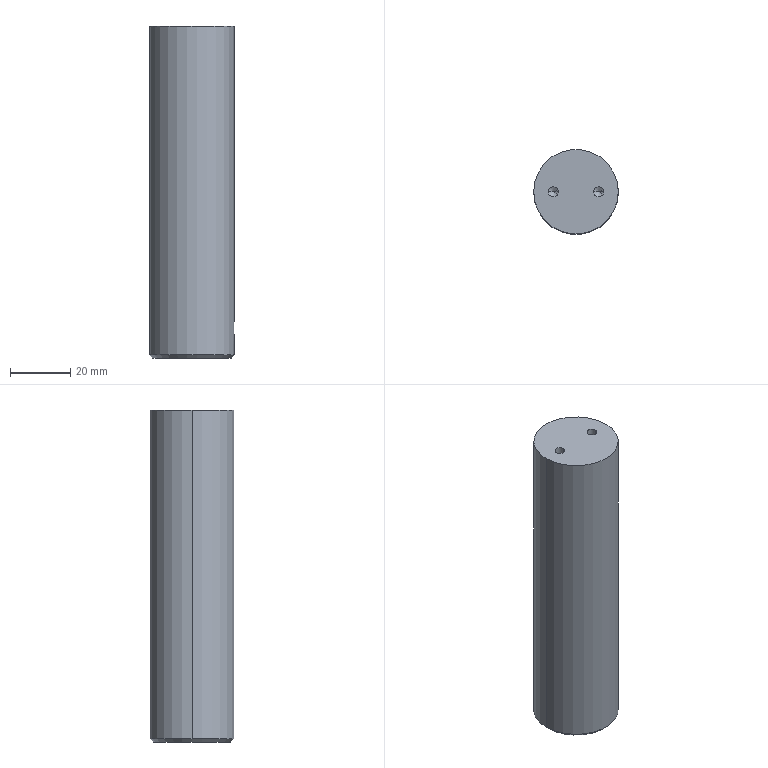Part | SolidWorks | features 3DProfileFeature 2, HoleWzd 2, Chamfer 1, Revolution 1 | 1 solid | 21 faces | box 28 x 28 x 110 mm | volume 51946 mm3 | cylinder 10 | cone 8 | plane 3 | commonest cylinder face diameters 3.3 x4 5 x2 18.1 x2 28 x2
STEP:
#1=CARTESIAN_POINT('',(9.05,0.,-109.));
#2=VERTEX_POINT('',#1);
#3=CARTESIAN_POINT('',(-9.05,0.,-109.));
#4=VERTEX_POINT('',#3);
#5=CARTESIAN_POINT('',(0.,0.,-109.));
#6=DIRECTION('',(0.,0.,-1.));
#7=DIRECTION('',(-1.,0.,0.));
#8=AXIS2_PLACEMENT_3D('',#5,#6,#7);
#9=CIRCLE('',#8,9.05);
#10=EDGE_CURVE('',#2,#4,#9,.T.);
#11=ORIENTED_EDGE('',*,*,#10,.F.);
#12=CARTESIAN_POINT('',(10.05,0.,-110.));
#13=VERTEX_POINT('',#12);
#14=CARTESIAN_POINT('',(9.05,0.,-109.));
#15=DIRECTION('',(0.7071,0.,-0.7071));
#16=VECTOR('',#15,1000.);
#17=LINE('',#14,#16);
#18=EDGE_CURVE('',#2,#13,#17,.T.);
#19=ORIENTED_EDGE('',*,*,#18,.T.);
#20=CARTESIAN_POINT('',(-10.05,0.,-110.));
#21=VERTEX_POINT('',#20);
#22=CARTESIAN_POINT('',(0.,0.,-110.));
#23=DIRECTION('',(0.,0.,1.));
#24=DIRECTION('',(-1.,0.,0.));
#25=AXIS2_PLACEMENT_3D('',#22,#23,#24);
#26=CIRCLE('',#25,10.05);
#27=EDGE_CURVE('',#21,#13,#26,.T.);
#28=ORIENTED_EDGE('',*,*,#27,.F.);
#29=CARTESIAN_POINT('',(-9.05,0.,-109.));
#30=DIRECTION('',(-0.7071,0.,-0.7071));
#31=VECTOR('',#30,1000.);
#32=LINE('',#29,#31);
#33=EDGE_CURVE('',#4,#21,#32,.T.);
#34=ORIENTED_EDGE('',*,*,#33,.F.);
#35=EDGE_LOOP('',(#11,#19,#28,#34));
#36=FACE_OUTER_BOUND('',#35,.T.);
#37=CARTESIAN_POINT('',(0.,0.,-109.));
#38=DIRECTION('',(0.,0.,-1.));
#39=DIRECTION('',(-1.,0.,0.));
#40=AXIS2_PLACEMENT_3D('',#37,#38,#39);
#41=CONICAL_SURFACE('',#40,9.05,0.7854);
#42=ADVANCED_FACE('',(#36),#41,.F.);
#43=CARTESIAN_POINT('',(-13.,0.,-110.));
#44=VERTEX_POINT('',#43);
#45=CARTESIAN_POINT('',(13.,0.,-110.));
#46=VERTEX_POINT('',#45);
#47=CARTESIAN_POINT('',(0.,0.,-110.));
#48=DIRECTION('',(0.,0.,-1.));
#49=DIRECTION('',(-1.,0.,0.));
#50=AXIS2_PLACEMENT_3D('',#47,#48,#49);
#51=CIRCLE('',#50,13.);
#52=EDGE_CURVE('',#44,#46,#51,.T.);
#53=ORIENTED_EDGE('',*,*,#52,.F.);
#54=CARTESIAN_POINT('',(-14.,0.,-109.));
#55=VERTEX_POINT('',#54);
#56=CARTESIAN_POINT('',(-13.,0.,-110.));
#57=DIRECTION('',(-0.7071,0.,0.7071));
#58=VECTOR('',#57,1000.);
#59=LINE('',#56,#58);
#60=EDGE_CURVE('',#44,#55,#59,.T.);
#61=ORIENTED_EDGE('',*,*,#60,.T.);
#62=CARTESIAN_POINT('',(14.,0.,-109.));
#63=VERTEX_POINT('',#62);
#64=CARTESIAN_POINT('',(0.,0.,-109.));
#65=DIRECTION('',(0.,0.,1.));
#66=DIRECTION('',(-1.,0.,0.));
#67=AXIS2_PLACEMENT_3D('',#64,#65,#66);
#68=CIRCLE('',#67,14.);
#69=EDGE_CURVE('',#63,#55,#68,.T.);
#70=ORIENTED_EDGE('',*,*,#69,.F.);
#71=CARTESIAN_POINT('',(13.,0.,-110.));
#72=DIRECTION('',(0.7071,0.,0.7071));
#73=VECTOR('',#72,1000.);
#74=LINE('',#71,#73);
#75=EDGE_CURVE('',#46,#63,#74,.T.);
#76=ORIENTED_EDGE('',*,*,#75,.F.);
#77=EDGE_LOOP('',(#53,#61,#70,#76));
#78=FACE_OUTER_BOUND('',#77,.T.);
#79=CARTESIAN_POINT('',(0.,0.,-110.));
#80=DIRECTION('',(0.,0.,1.));
#81=DIRECTION('',(1.,0.,0.));
#82=AXIS2_PLACEMENT_3D('',#79,#80,#81);
#83=CONICAL_SURFACE('',#82,13.,0.7854);
#84=ADVANCED_FACE('',(#78),#83,.T.);
#85=CARTESIAN_POINT('',(9.05,0.,-102.5));
#86=VERTEX_POINT('',#85);
#87=CARTESIAN_POINT('',(9.05,0.,-97.5));
#88=VERTEX_POINT('',#87);
#89=CARTESIAN_POINT('',(9.05,0.,-102.5));
#90=CARTESIAN_POINT('',(9.05,-0.1661,-102.5));
#91=CARTESIAN_POINT('',(9.045,-0.3292,-102.484));
#92=CARTESIAN_POINT('',(9.028,-0.6498,-102.42));
#93=CARTESIAN_POINT('',(9.015,-0.8091,-102.371));
#94=CARTESIAN_POINT('',(8.983,-1.112,-102.245));
#95=CARTESIAN_POINT('',(8.964,-1.255,-102.168));
#96=CARTESIAN_POINT('',(8.921,-1.526,-101.987));
#97=CARTESIAN_POINT('',(8.898,-1.654,-101.882));
#98=CARTESIAN_POINT('',(8.83,-1.998,-101.538));
#99=CARTESIAN_POINT('',(8.784,-2.184,-101.26));
#100=CARTESIAN_POINT('',(8.734,-2.371,-100.809));
#101=CARTESIAN_POINT('',(8.721,-2.419,-100.651));
#102=CARTESIAN_POINT('',(8.703,-2.484,-100.328));
#103=CARTESIAN_POINT('',(8.698,-2.5,-100.165));
#104=CARTESIAN_POINT('',(8.698,-2.5,-99.837));
#105=CARTESIAN_POINT('',(8.703,-2.484,-99.671));
#106=CARTESIAN_POINT('',(8.721,-2.419,-99.349));
#107=CARTESIAN_POINT('',(8.734,-2.372,-99.193));
#108=CARTESIAN_POINT('',(8.784,-2.183,-98.737));
#109=CARTESIAN_POINT('',(8.83,-1.999,-98.463));
#110=CARTESIAN_POINT('',(8.899,-1.652,-98.116));
#111=CARTESIAN_POINT('',(8.921,-1.526,-98.013));
#112=CARTESIAN_POINT('',(8.963,-1.256,-97.832));
#113=CARTESIAN_POINT('',(8.983,-1.11,-97.754));
#114=CARTESIAN_POINT('',(9.015,-0.808,-97.629));
#115=CARTESIAN_POINT('',(9.028,-0.6521,-97.581));
#116=CARTESIAN_POINT('',(9.045,-0.3296,-97.516));
#117=CARTESIAN_POINT('',(9.05,-0.1637,-97.5));
#118=CARTESIAN_POINT('',(9.05,0.,-97.5));
#119=B_SPLINE_CURVE_WITH_KNOTS('',3,(#89,#90,#91,#92,#93,#94,#95,#96,#97,#98,#99,#100,#101,#102,#103,#104,#105,#106,#107,#108,#109,#110,#111,#112,#113,#114,#115,#116,#117,#118),.UNSPECIFIED.,.F.,.F.,(4,2,2,2,2,2,2,2,2,2,2,2,2,2,4),(0.,0.0004909,0.0009818,0.001473,0.001964,0.002945,0.003436,0.003927,0.004418,0.004909,0.005891,0.006382,0.006873,0.007364,0.007855),.UNSPECIFIED.);
#120=EDGE_CURVE('',#86,#88,#119,.T.);
#121=ORIENTED_EDGE('',*,*,#120,.T.);
#122=CARTESIAN_POINT('',(14.,0.,-97.5));
#123=VERTEX_POINT('',#122);
#124=CARTESIAN_POINT('',(14.,0.,-97.5));
#125=DIRECTION('',(1.,0.,0.));
#126=VECTOR('',#125,1000.);
#127=LINE('',#124,#126);
#128=EDGE_CURVE('',#88,#123,#127,.T.);
#129=ORIENTED_EDGE('',*,*,#128,.T.);
#130=CARTESIAN_POINT('',(14.,0.,-102.5));
#131=VERTEX_POINT('',#130);
#132=CARTESIAN_POINT('',(14.,0.,-97.5));
#133=CARTESIAN_POINT('',(14.,-0.3266,-97.5));
#134=CARTESIAN_POINT('',(13.988,-0.6561,-97.566));
#135=CARTESIAN_POINT('',(13.957,-1.108,-97.753));
#136=CARTESIAN_POINT('',(13.944,-1.253,-97.831));
#137=CARTESIAN_POINT('',(13.917,-1.526,-98.013));
#138=CARTESIAN_POINT('',(13.903,-1.651,-98.116));
#139=CARTESIAN_POINT('',(13.873,-1.882,-98.346));
#140=CARTESIAN_POINT('',(13.859,-1.987,-98.475));
#141=CARTESIAN_POINT('',(13.831,-2.169,-98.745));
#142=CARTESIAN_POINT('',(13.819,-2.246,-98.889));
#143=CARTESIAN_POINT('',(13.798,-2.371,-99.192));
#144=CARTESIAN_POINT('',(13.789,-2.42,-99.35));
#145=CARTESIAN_POINT('',(13.778,-2.483,-99.67));
#146=CARTESIAN_POINT('',(13.775,-2.5,-99.833));
#147=CARTESIAN_POINT('',(13.775,-2.5,-100.164));
#148=CARTESIAN_POINT('',(13.778,-2.484,-100.326));
#149=CARTESIAN_POINT('',(13.789,-2.42,-100.646));
#150=CARTESIAN_POINT('',(13.798,-2.372,-100.806));
#151=CARTESIAN_POINT('',(13.819,-2.247,-101.108));
#152=CARTESIAN_POINT('',(13.831,-2.17,-101.251));
#153=CARTESIAN_POINT('',(13.858,-1.989,-101.523));
#154=CARTESIAN_POINT('',(13.873,-1.884,-101.652));
#155=CARTESIAN_POINT('',(13.917,-1.539,-101.997));
#156=CARTESIAN_POINT('',(13.946,-1.261,-102.183));
#157=CARTESIAN_POINT('',(13.977,-0.81,-102.371));
#158=CARTESIAN_POINT('',(13.986,-0.6517,-102.419));
#159=CARTESIAN_POINT('',(13.997,-0.3289,-102.484));
#160=CARTESIAN_POINT('',(14.,-0.1655,-102.5));
#161=CARTESIAN_POINT('',(14.,0.,-102.5));
#162=B_SPLINE_CURVE_WITH_KNOTS('',3,(#132,#133,#134,#135,#136,#137,#138,#139,#140,#141,#142,#143,#144,#145,#146,#147,#148,#149,#150,#151,#152,#153,#154,#155,#156,#157,#158,#159,#160,#161),.UNSPECIFIED.,.F.,.F.,(4,2,2,2,2,2,2,2,2,2,2,2,2,2,4),(0.007832,0.008811,0.0093,0.009789,0.01028,0.01077,0.01126,0.01175,0.01224,0.01273,0.01321,0.0137,0.01468,0.01517,0.01566),.UNSPECIFIED.);
#163=EDGE_CURVE('',#123,#131,#162,.T.);
#164=ORIENTED_EDGE('',*,*,#163,.T.);
#165=CARTESIAN_POINT('',(14.,0.,-102.5));
#166=DIRECTION('',(1.,0.,0.));
#167=VECTOR('',#166,1000.);
#168=LINE('',#165,#167);
#169=EDGE_CURVE('',#86,#131,#168,.T.);
#170=ORIENTED_EDGE('',*,*,#169,.F.);
#171=EDGE_LOOP('',(#121,#129,#164,#170));
#172=FACE_OUTER_BOUND('',#171,.T.);
#173=CARTESIAN_POINT('',(14.,0.,-100.));
#174=DIRECTION('',(1.,0.,0.));
#175=DIRECTION('',(0.,0.,-1.));
#176=AXIS2_PLACEMENT_3D('',#173,#174,#175);
#177=CYLINDRICAL_SURFACE('',#176,2.5);
#178=ADVANCED_FACE('',(#172),#177,.F.);
#179=CARTESIAN_POINT('',(-9.15,0.,-10.1));
#180=VERTEX_POINT('',#179);
#181=CARTESIAN_POINT('',(-5.85,0.,-10.1));
#182=VERTEX_POINT('',#181);
#183=CARTESIAN_POINT('',(-7.5,0.,-10.1));
#184=DIRECTION('',(0.,0.,1.));
#185=DIRECTION('',(1.,0.,0.));
#186=AXIS2_PLACEMENT_3D('',#183,#184,#185);
#187=CIRCLE('',#186,1.65);
#188=EDGE_CURVE('',#180,#182,#187,.T.);
#189=ORIENTED_EDGE('',*,*,#188,.F.);
#190=CARTESIAN_POINT('',(-9.15,0.,0.));
#191=VERTEX_POINT('',#190);
#192=CARTESIAN_POINT('',(-9.15,0.,0.));
#193=DIRECTION('',(0.,0.,1.));
#194=VECTOR('',#193,1000.);
#195=LINE('',#192,#194);
#196=EDGE_CURVE('',#180,#191,#195,.T.);
#197=ORIENTED_EDGE('',*,*,#196,.T.);
#198=CARTESIAN_POINT('',(-5.85,0.,0.));
#199=VERTEX_POINT('',#198);
#200=CARTESIAN_POINT('',(-7.5,0.,0.));
#201=DIRECTION('',(0.,0.,1.));
#202=DIRECTION('',(1.,0.,0.));
#203=AXIS2_PLACEMENT_3D('',#200,#201,#202);
#204=CIRCLE('',#203,1.65);
#205=EDGE_CURVE('',#191,#199,#204,.T.);
#206=ORIENTED_EDGE('',*,*,#205,.T.);
#207=CARTESIAN_POINT('',(-5.85,0.,0.));
#208=DIRECTION('',(0.,0.,1.));
#209=VECTOR('',#208,1000.);
#210=LINE('',#207,#209);
#211=EDGE_CURVE('',#182,#199,#210,.T.);
#212=ORIENTED_EDGE('',*,*,#211,.F.);
#213=EDGE_LOOP('',(#189,#197,#206,#212));
#214=FACE_OUTER_BOUND('',#213,.T.);
#215=CARTESIAN_POINT('',(-7.5,0.,0.));
#216=DIRECTION('',(0.,0.,1.));
#217=DIRECTION('',(1.,0.,0.));
#218=AXIS2_PLACEMENT_3D('',#215,#216,#217);
#219=CYLINDRICAL_SURFACE('',#218,1.65);
#220=ADVANCED_FACE('',(#214),#219,.F.);
#221=CARTESIAN_POINT('',(-7.5,0.,-11.091));
#222=VERTEX_POINT('',#221);
#223=CARTESIAN_POINT('',(-5.85,0.,-10.1));
#224=DIRECTION('',(0.8572,0.,0.515));
#225=VECTOR('',#224,1000.);
#226=LINE('',#223,#225);
#227=EDGE_CURVE('',#222,#182,#226,.T.);
#228=ORIENTED_EDGE('',*,*,#227,.F.);
#229=CARTESIAN_POINT('',(-9.15,0.,-10.1));
#230=DIRECTION('',(-0.8572,0.,0.515));
#231=VECTOR('',#230,1000.);
#232=LINE('',#229,#231);
#233=EDGE_CURVE('',#222,#180,#232,.T.);
#234=ORIENTED_EDGE('',*,*,#233,.T.);
#235=ORIENTED_EDGE('',*,*,#188,.T.);
#236=EDGE_LOOP('',(#228,#234,#235));
#237=FACE_OUTER_BOUND('',#236,.T.);
#238=CARTESIAN_POINT('',(-7.5,0.,-10.1));
#239=DIRECTION('',(0.,0.,1.));
#240=DIRECTION('',(1.,0.,0.));
#241=AXIS2_PLACEMENT_3D('',#238,#239,#240);
#242=CONICAL_SURFACE('',#241,1.65,1.03);
#243=ADVANCED_FACE('',(#237),#242,.F.);
#244=CARTESIAN_POINT('',(5.85,0.,-10.1));
#245=VERTEX_POINT('',#244);
#246=CARTESIAN_POINT('',(9.15,0.,-10.1));
#247=VERTEX_POINT('',#246);
#248=CARTESIAN_POINT('',(7.5,0.,-10.1));
#249=DIRECTION('',(0.,0.,1.));
#250=DIRECTION('',(1.,0.,0.));
#251=AXIS2_PLACEMENT_3D('',#248,#249,#250);
#252=CIRCLE('',#251,1.65);
#253=EDGE_CURVE('',#245,#247,#252,.T.);
#254=ORIENTED_EDGE('',*,*,#253,.F.);
#255=CARTESIAN_POINT('',(5.85,0.,0.));
#256=VERTEX_POINT('',#255);
#257=CARTESIAN_POINT('',(5.85,0.,0.));
#258=DIRECTION('',(0.,0.,1.));
#259=VECTOR('',#258,1000.);
#260=LINE('',#257,#259);
#261=EDGE_CURVE('',#245,#256,#260,.T.);
#262=ORIENTED_EDGE('',*,*,#261,.T.);
#263=CARTESIAN_POINT('',(9.15,0.,0.));
#264=VERTEX_POINT('',#263);
#265=CARTESIAN_POINT('',(7.5,0.,0.));
#266=DIRECTION('',(0.,0.,1.));
#267=DIRECTION('',(1.,0.,0.));
#268=AXIS2_PLACEMENT_3D('',#265,#266,#267);
#269=CIRCLE('',#268,1.65);
#270=EDGE_CURVE('',#256,#264,#269,.T.);
#271=ORIENTED_EDGE('',*,*,#270,.T.);
#272=CARTESIAN_POINT('',(9.15,0.,0.));
#273=DIRECTION('',(0.,0.,1.));
#274=VECTOR('',#273,1000.);
#275=LINE('',#272,#274);
#276=EDGE_CURVE('',#247,#264,#275,.T.);
#277=ORIENTED_EDGE('',*,*,#276,.F.);
#278=EDGE_LOOP('',(#254,#262,#271,#277));
#279=FACE_OUTER_BOUND('',#278,.T.);
#280=CARTESIAN_POINT('',(7.5,0.,0.));
#281=DIRECTION('',(0.,0.,1.));
#282=DIRECTION('',(1.,0.,0.));
#283=AXIS2_PLACEMENT_3D('',#280,#281,#282);
#284=CYLINDRICAL_SURFACE('',#283,1.65);
#285=ADVANCED_FACE('',(#279),#284,.F.);
#286=CARTESIAN_POINT('',(7.5,0.,-11.091));
#287=VERTEX_POINT('',#286);
#288=CARTESIAN_POINT('',(9.15,0.,-10.1));
#289=DIRECTION('',(0.8572,0.,0.515));
#290=VECTOR('',#289,1000.);
#291=LINE('',#288,#290);
#292=EDGE_CURVE('',#287,#247,#291,.T.);
#293=ORIENTED_EDGE('',*,*,#292,.F.);
#294=CARTESIAN_POINT('',(5.85,0.,-10.1));
#295=DIRECTION('',(-0.8572,0.,0.515));
#296=VECTOR('',#295,1000.);
#297=LINE('',#294,#296);
#298=EDGE_CURVE('',#287,#245,#297,.T.);
#299=ORIENTED_EDGE('',*,*,#298,.T.);
#300=ORIENTED_EDGE('',*,*,#253,.T.);
#301=EDGE_LOOP('',(#293,#299,#300));
#302=FACE_OUTER_BOUND('',#301,.T.);
#303=CARTESIAN_POINT('',(7.5,0.,-10.1));
#304=DIRECTION('',(0.,0.,1.));
#305=DIRECTION('',(1.,0.,0.));
#306=AXIS2_PLACEMENT_3D('',#303,#304,#305);
#307=CONICAL_SURFACE('',#306,1.65,1.03);
#308=ADVANCED_FACE('',(#302),#307,.F.);
#309=CARTESIAN_POINT('',(9.05,0.,-50.));
#310=VERTEX_POINT('',#309);
#311=CARTESIAN_POINT('',(-9.05,0.,-50.));
#312=VERTEX_POINT('',#311);
#313=CARTESIAN_POINT('',(0.,0.,-50.));
#314=DIRECTION('',(0.,0.,-1.));
#315=DIRECTION('',(-1.,0.,0.));
#316=AXIS2_PLACEMENT_3D('',#313,#314,#315);
#317=CIRCLE('',#316,9.05);
#318=EDGE_CURVE('',#310,#312,#317,.T.);
#319=ORIENTED_EDGE('',*,*,#318,.F.);
#320=CARTESIAN_POINT('',(9.05,0.,-50.));
#321=DIRECTION('',(0.,0.,-1.));
#322=VECTOR('',#321,1000.);
#323=LINE('',#320,#322);
#324=EDGE_CURVE('',#310,#88,#323,.T.);
#325=ORIENTED_EDGE('',*,*,#324,.T.);
#326=ORIENTED_EDGE('',*,*,#120,.F.);
#327=CARTESIAN_POINT('',(9.05,0.,-50.));
#328=DIRECTION('',(0.,0.,-1.));
#329=VECTOR('',#328,1000.);
#330=LINE('',#327,#329);
#331=EDGE_CURVE('',#86,#2,#330,.T.);
#332=ORIENTED_EDGE('',*,*,#331,.T.);
#333=ORIENTED_EDGE('',*,*,#10,.T.);
#334=CARTESIAN_POINT('',(-9.05,0.,-50.));
#335=DIRECTION('',(0.,0.,-1.));
#336=VECTOR('',#335,1000.);
#337=LINE('',#334,#336);
#338=EDGE_CURVE('',#312,#4,#337,.T.);
#339=ORIENTED_EDGE('',*,*,#338,.F.);
#340=EDGE_LOOP('',(#319,#325,#326,#332,#333,#339));
#341=FACE_OUTER_BOUND('',#340,.T.);
#342=CARTESIAN_POINT('',(0.,0.,-50.));
#343=DIRECTION('',(0.,0.,-1.));
#344=DIRECTION('',(-1.,0.,0.));
#345=AXIS2_PLACEMENT_3D('',#342,#343,#344);
#346=CYLINDRICAL_SURFACE('',#345,9.05);
#347=ADVANCED_FACE('',(#341),#346,.F.);
#348=CARTESIAN_POINT('',(-14.,0.,0.));
#349=VERTEX_POINT('',#348);
#350=CARTESIAN_POINT('',(14.,0.,0.));
#351=VERTEX_POINT('',#350);
#352=CARTESIAN_POINT('',(0.,0.,0.));
#353=DIRECTION('',(0.,0.,-1.));
#354=DIRECTION('',(-1.,0.,0.));
#355=AXIS2_PLACEMENT_3D('',#352,#353,#354);
#356=CIRCLE('',#355,14.);
#357=EDGE_CURVE('',#349,#351,#356,.T.);
#358=ORIENTED_EDGE('',*,*,#357,.T.);
#359=CARTESIAN_POINT('',(14.,0.,-50.));
#360=DIRECTION('',(0.,0.,-1.));
#361=VECTOR('',#360,1000.);
#362=LINE('',#359,#361);
#363=EDGE_CURVE('',#351,#123,#362,.T.);
#364=ORIENTED_EDGE('',*,*,#363,.T.);
#365=CARTESIAN_POINT('',(14.,0.,-102.5));
#366=CARTESIAN_POINT('',(14.,0.1655,-102.5));
#367=CARTESIAN_POINT('',(13.997,0.3282,-102.484));
#368=CARTESIAN_POINT('',(13.986,0.6482,-102.42));
#369=CARTESIAN_POINT('',(13.978,0.8072,-102.372));
#370=CARTESIAN_POINT('',(13.957,1.11,-102.246));
#371=CARTESIAN_POINT('',(13.944,1.253,-102.169));
#372=CARTESIAN_POINT('',(13.917,1.525,-101.988));
#373=CARTESIAN_POINT('',(13.903,1.653,-101.882));
#374=CARTESIAN_POINT('',(13.859,1.998,-101.537));
#375=CARTESIAN_POINT('',(13.829,2.184,-101.259));
#376=CARTESIAN_POINT('',(13.798,2.372,-100.808));
#377=CARTESIAN_POINT('',(13.789,2.42,-100.65));
#378=CARTESIAN_POINT('',(13.778,2.484,-100.327));
#379=CARTESIAN_POINT('',(13.775,2.5,-100.164));
#380=CARTESIAN_POINT('',(13.775,2.5,-99.838));
#381=CARTESIAN_POINT('',(13.778,2.484,-99.671));
#382=CARTESIAN_POINT('',(13.789,2.42,-99.351));
#383=CARTESIAN_POINT('',(13.798,2.372,-99.195));
#384=CARTESIAN_POINT('',(13.819,2.247,-98.891));
#385=CARTESIAN_POINT('',(13.831,2.169,-98.746));
#386=CARTESIAN_POINT('',(13.858,1.988,-98.475));
#387=CARTESIAN_POINT('',(13.873,1.884,-98.349));
#388=CARTESIAN_POINT('',(13.903,1.651,-98.116));
#389=CARTESIAN_POINT('',(13.917,1.525,-98.013));
#390=CARTESIAN_POINT('',(13.944,1.255,-97.832));
#391=CARTESIAN_POINT('',(13.957,1.109,-97.753));
#392=CARTESIAN_POINT('',(13.978,0.8062,-97.628));
#393=CARTESIAN_POINT('',(13.986,0.6504,-97.581));
#394=CARTESIAN_POINT('',(13.997,0.3293,-97.516));
#395=CARTESIAN_POINT('',(14.,0.1633,-97.5));
#396=CARTESIAN_POINT('',(14.,0.,-97.5));
#397=B_SPLINE_CURVE_WITH_KNOTS('',3,(#365,#366,#367,#368,#369,#370,#371,#372,#373,#374,#375,#376,#377,#378,#379,#380,#381,#382,#383,#384,#385,#386,#387,#388,#389,#390,#391,#392,#393,#394,#395,#396),.UNSPECIFIED.,.F.,.F.,(4,2,2,2,2,2,2,2,2,2,2,2,2,2,2,4),(0.,0.0004895,0.000979,0.001468,0.001958,0.002937,0.003426,0.003916,0.004405,0.004895,0.005384,0.005874,0.006363,0.006853,0.007342,0.007832),.UNSPECIFIED.);
#398=EDGE_CURVE('',#131,#123,#397,.T.);
#399=ORIENTED_EDGE('',*,*,#398,.F.);
#400=CARTESIAN_POINT('',(14.,0.,-50.));
#401=DIRECTION('',(0.,0.,-1.));
#402=VECTOR('',#401,1000.);
#403=LINE('',#400,#402);
#404=EDGE_CURVE('',#131,#63,#403,.T.);
#405=ORIENTED_EDGE('',*,*,#404,.T.);
#406=ORIENTED_EDGE('',*,*,#69,.T.);
#407=CARTESIAN_POINT('',(-14.,0.,-50.));
#408=DIRECTION('',(0.,0.,-1.));
#409=VECTOR('',#408,1000.);
#410=LINE('',#407,#409);
#411=EDGE_CURVE('',#349,#55,#410,.T.);
#412=ORIENTED_EDGE('',*,*,#411,.F.);
#413=EDGE_LOOP('',(#358,#364,#399,#405,#406,#412));
#414=FACE_OUTER_BOUND('',#413,.T.);
#415=CARTESIAN_POINT('',(0.,0.,-50.));
#416=DIRECTION('',(0.,0.,-1.));
#417=DIRECTION('',(-1.,0.,0.));
#418=AXIS2_PLACEMENT_3D('',#415,#416,#417);
#419=CYLINDRICAL_SURFACE('',#418,14.);
#420=ADVANCED_FACE('',(#414),#419,.T.);
#421=ORIENTED_EDGE('',*,*,#363,.F.);
#422=CARTESIAN_POINT('',(0.,0.,0.));
#423=DIRECTION('',(0.,0.,-1.));
#424=DIRECTION('',(-1.,0.,0.));
#425=AXIS2_PLACEMENT_3D('',#422,#423,#424);
#426=CIRCLE('',#425,14.);
#427=EDGE_CURVE('',#351,#349,#426,.T.);
#428=ORIENTED_EDGE('',*,*,#427,.T.);
#429=ORIENTED_EDGE('',*,*,#411,.T.);
#430=CARTESIAN_POINT('',(0.,0.,-109.));
#431=DIRECTION('',(0.,0.,1.));
#432=DIRECTION('',(-1.,0.,0.));
#433=AXIS2_PLACEMENT_3D('',#430,#431,#432);
#434=CIRCLE('',#433,14.);
#435=EDGE_CURVE('',#55,#63,#434,.T.);
#436=ORIENTED_EDGE('',*,*,#435,.T.);
#437=ORIENTED_EDGE('',*,*,#404,.F.);
#438=ORIENTED_EDGE('',*,*,#163,.F.);
#439=EDGE_LOOP('',(#421,#428,#429,#436,#437,#438));
#440=FACE_OUTER_BOUND('',#439,.T.);
#441=CARTESIAN_POINT('',(0.,0.,-50.));
#442=DIRECTION('',(0.,0.,-1.));
#443=DIRECTION('',(-1.,0.,0.));
#444=AXIS2_PLACEMENT_3D('',#441,#442,#443);
#445=CYLINDRICAL_SURFACE('',#444,14.);
#446=ADVANCED_FACE('',(#440),#445,.T.);
#447=CARTESIAN_POINT('',(-7.5,0.,0.));
#448=DIRECTION('',(0.,0.,1.));
#449=DIRECTION('',(1.,0.,0.));
#450=AXIS2_PLACEMENT_3D('',#447,#448,#449);
#451=CIRCLE('',#450,1.65);
#452=EDGE_CURVE('',#199,#191,#451,.T.);
#453=ORIENTED_EDGE('',*,*,#452,.F.);
#454=ORIENTED_EDGE('',*,*,#205,.F.);
#455=EDGE_LOOP('',(#453,#454));
#456=FACE_BOUND('',#455,.T.);
#457=CARTESIAN_POINT('',(7.5,0.,0.));
#458=DIRECTION('',(0.,0.,1.));
#459=DIRECTION('',(1.,0.,0.));
#460=AXIS2_PLACEMENT_3D('',#457,#458,#459);
#461=CIRCLE('',#460,1.65);
#462=EDGE_CURVE('',#264,#256,#461,.T.);
#463=ORIENTED_EDGE('',*,*,#462,.F.);
#464=ORIENTED_EDGE('',*,*,#270,.F.);
#465=EDGE_LOOP('',(#463,#464));
#466=FACE_BOUND('',#465,.T.);
#467=ORIENTED_EDGE('',*,*,#357,.F.);
#468=ORIENTED_EDGE('',*,*,#427,.F.);
#469=EDGE_LOOP('',(#467,#468));
#470=FACE_OUTER_BOUND('',#469,.T.);
#471=CARTESIAN_POINT('',(-14.,0.,0.));
#472=DIRECTION('',(0.,0.,1.));
#473=DIRECTION('',(1.,0.,0.));
#474=AXIS2_PLACEMENT_3D('',#471,#472,#473);
#475=PLANE('',#474);
#476=ADVANCED_FACE('',(#456,#466,#470),#475,.T.);
#477=CARTESIAN_POINT('',(0.,0.,-50.));
#478=DIRECTION('',(0.,0.,-1.));
#479=DIRECTION('',(-1.,0.,0.));
#480=AXIS2_PLACEMENT_3D('',#477,#478,#479);
#481=CIRCLE('',#480,9.05);
#482=EDGE_CURVE('',#312,#310,#481,.T.);
#483=ORIENTED_EDGE('',*,*,#482,.T.);
#484=ORIENTED_EDGE('',*,*,#318,.T.);
#485=EDGE_LOOP('',(#483,#484));
#486=FACE_OUTER_BOUND('',#485,.T.);
#487=CARTESIAN_POINT('',(-9.05,0.,-50.));
#488=DIRECTION('',(0.,0.,-1.));
#489=DIRECTION('',(-1.,0.,0.));
#490=AXIS2_PLACEMENT_3D('',#487,#488,#489);
#491=PLANE('',#490);
#492=ADVANCED_FACE('',(#486),#491,.T.);
#493=ORIENTED_EDGE('',*,*,#324,.F.);
#494=ORIENTED_EDGE('',*,*,#482,.F.);
#495=ORIENTED_EDGE('',*,*,#338,.T.);
#496=CARTESIAN_POINT('',(0.,0.,-109.));
#497=DIRECTION('',(0.,0.,-1.));
#498=DIRECTION('',(-1.,0.,0.));
#499=AXIS2_PLACEMENT_3D('',#496,#497,#498);
#500=CIRCLE('',#499,9.05);
#501=EDGE_CURVE('',#4,#2,#500,.T.);
#502=ORIENTED_EDGE('',*,*,#501,.T.);
#503=ORIENTED_EDGE('',*,*,#331,.F.);
#504=CARTESIAN_POINT('',(9.05,0.,-97.5));
#505=CARTESIAN_POINT('',(9.05,0.3272,-97.5));
#506=CARTESIAN_POINT('',(9.031,0.6577,-97.566));
#507=CARTESIAN_POINT('',(8.983,1.11,-97.754));
#508=CARTESIAN_POINT('',(8.963,1.256,-97.832));
#509=CARTESIAN_POINT('',(8.921,1.527,-98.014));
#510=CARTESIAN_POINT('',(8.899,1.652,-98.116));
#511=CARTESIAN_POINT('',(8.853,1.883,-98.347));
#512=CARTESIAN_POINT('',(8.83,1.987,-98.475));
#513=CARTESIAN_POINT('',(8.787,2.168,-98.744));
#514=CARTESIAN_POINT('',(8.767,2.245,-98.888));
#515=CARTESIAN_POINT('',(8.734,2.372,-99.192));
#516=CARTESIAN_POINT('',(8.721,2.419,-99.349));
#517=CARTESIAN_POINT('',(8.703,2.483,-99.669));
#518=CARTESIAN_POINT('',(8.698,2.5,-99.835));
#519=CARTESIAN_POINT('',(8.698,2.5,-100.164));
#520=CARTESIAN_POINT('',(8.703,2.484,-100.327));
#521=CARTESIAN_POINT('',(8.721,2.42,-100.649));
#522=CARTESIAN_POINT('',(8.734,2.371,-100.808));
#523=CARTESIAN_POINT('',(8.784,2.184,-101.26));
#524=CARTESIAN_POINT('',(8.83,1.998,-101.538));
#525=CARTESIAN_POINT('',(8.898,1.654,-101.882));
#526=CARTESIAN_POINT('',(8.921,1.527,-101.986));
#527=CARTESIAN_POINT('',(8.964,1.255,-102.168));
#528=CARTESIAN_POINT('',(8.983,1.112,-102.245));
#529=CARTESIAN_POINT('',(9.015,0.8109,-102.37));
#530=CARTESIAN_POINT('',(9.028,0.6513,-102.419));
#531=CARTESIAN_POINT('',(9.045,0.3295,-102.484));
#532=CARTESIAN_POINT('',(9.05,0.166,-102.5));
#533=CARTESIAN_POINT('',(9.05,0.,-102.5));
#534=B_SPLINE_CURVE_WITH_KNOTS('',3,(#504,#505,#506,#507,#508,#509,#510,#511,#512,#513,#514,#515,#516,#517,#518,#519,#520,#521,#522,#523,#524,#525,#526,#527,#528,#529,#530,#531,#532,#533),.UNSPECIFIED.,.F.,.F.,(4,2,2,2,2,2,2,2,2,2,2,2,2,2,4),(0.007855,0.008836,0.009327,0.009818,0.01031,0.0108,0.01129,0.01178,0.01227,0.01276,0.01374,0.01423,0.01473,0.01522,0.01571),.UNSPECIFIED.);
#535=EDGE_CURVE('',#88,#86,#534,.T.);
#536=ORIENTED_EDGE('',*,*,#535,.F.);
#537=EDGE_LOOP('',(#493,#494,#495,#502,#503,#536));
#538=FACE_OUTER_BOUND('',#537,.T.);
#539=CARTESIAN_POINT('',(0.,0.,-50.));
#540=DIRECTION('',(0.,0.,-1.));
#541=DIRECTION('',(-1.,0.,0.));
#542=AXIS2_PLACEMENT_3D('',#539,#540,#541);
#543=CYLINDRICAL_SURFACE('',#542,9.05);
#544=ADVANCED_FACE('',(#538),#543,.F.);
#545=CARTESIAN_POINT('',(0.,0.,-110.));
#546=DIRECTION('',(0.,0.,-1.));
#547=DIRECTION('',(-1.,0.,0.));
#548=AXIS2_PLACEMENT_3D('',#545,#546,#547);
#549=CIRCLE('',#548,13.);
#550=EDGE_CURVE('',#46,#44,#549,.T.);
#551=ORIENTED_EDGE('',*,*,#550,.T.);
#552=ORIENTED_EDGE('',*,*,#52,.T.);
#553=EDGE_LOOP('',(#551,#552));
#554=FACE_OUTER_BOUND('',#553,.T.);
#555=ORIENTED_EDGE('',*,*,#27,.T.);
#556=CARTESIAN_POINT('',(0.,0.,-110.));
#557=DIRECTION('',(0.,0.,1.));
#558=DIRECTION('',(-1.,0.,0.));
#559=AXIS2_PLACEMENT_3D('',#556,#557,#558);
#560=CIRCLE('',#559,10.05);
#561=EDGE_CURVE('',#13,#21,#560,.T.);
#562=ORIENTED_EDGE('',*,*,#561,.T.);
#563=EDGE_LOOP('',(#555,#562));
#564=FACE_BOUND('',#563,.T.);
#565=CARTESIAN_POINT('',(-9.05,0.,-110.));
#566=DIRECTION('',(0.,0.,-1.));
#567=DIRECTION('',(-1.,0.,0.));
#568=AXIS2_PLACEMENT_3D('',#565,#566,#567);
#569=PLANE('',#568);
#570=ADVANCED_FACE('',(#554,#564),#569,.T.);
#571=ORIENTED_EDGE('',*,*,#298,.F.);
#572=ORIENTED_EDGE('',*,*,#292,.T.);
#573=CARTESIAN_POINT('',(7.5,0.,-10.1));
#574=DIRECTION('',(0.,0.,1.));
#575=DIRECTION('',(1.,0.,0.));
#576=AXIS2_PLACEMENT_3D('',#573,#574,#575);
#577=CIRCLE('',#576,1.65);
#578=EDGE_CURVE('',#247,#245,#577,.T.);
#579=ORIENTED_EDGE('',*,*,#578,.T.);
#580=EDGE_LOOP('',(#571,#572,#579));
#581=FACE_OUTER_BOUND('',#580,.T.);
#582=CARTESIAN_POINT('',(7.5,0.,-10.1));
#583=DIRECTION('',(0.,0.,1.));
#584=DIRECTION('',(1.,0.,0.));
#585=AXIS2_PLACEMENT_3D('',#582,#583,#584);
#586=CONICAL_SURFACE('',#585,1.65,1.03);
#587=ADVANCED_FACE('',(#581),#586,.F.);
#588=ORIENTED_EDGE('',*,*,#261,.F.);
#589=ORIENTED_EDGE('',*,*,#578,.F.);
#590=ORIENTED_EDGE('',*,*,#276,.T.);
#591=ORIENTED_EDGE('',*,*,#462,.T.);
#592=EDGE_LOOP('',(#588,#589,#590,#591));
#593=FACE_OUTER_BOUND('',#592,.T.);
#594=CARTESIAN_POINT('',(7.5,0.,0.));
#595=DIRECTION('',(0.,0.,1.));
#596=DIRECTION('',(1.,0.,0.));
#597=AXIS2_PLACEMENT_3D('',#594,#595,#596);
#598=CYLINDRICAL_SURFACE('',#597,1.65);
#599=ADVANCED_FACE('',(#593),#598,.F.);
#600=ORIENTED_EDGE('',*,*,#233,.F.);
#601=ORIENTED_EDGE('',*,*,#227,.T.);
#602=CARTESIAN_POINT('',(-7.5,0.,-10.1));
#603=DIRECTION('',(0.,0.,1.));
#604=DIRECTION('',(1.,0.,0.));
#605=AXIS2_PLACEMENT_3D('',#602,#603,#604);
#606=CIRCLE('',#605,1.65);
#607=EDGE_CURVE('',#182,#180,#606,.T.);
#608=ORIENTED_EDGE('',*,*,#607,.T.);
#609=EDGE_LOOP('',(#600,#601,#608));
#610=FACE_OUTER_BOUND('',#609,.T.);
#611=CARTESIAN_POINT('',(-7.5,0.,-10.1));
#612=DIRECTION('',(0.,0.,1.));
#613=DIRECTION('',(1.,0.,0.));
#614=AXIS2_PLACEMENT_3D('',#611,#612,#613);
#615=CONICAL_SURFACE('',#614,1.65,1.03);
#616=ADVANCED_FACE('',(#610),#615,.F.);
#617=ORIENTED_EDGE('',*,*,#196,.F.);
#618=ORIENTED_EDGE('',*,*,#607,.F.);
#619=ORIENTED_EDGE('',*,*,#211,.T.);
#620=ORIENTED_EDGE('',*,*,#452,.T.);
#621=EDGE_LOOP('',(#617,#618,#619,#620));
#622=FACE_OUTER_BOUND('',#621,.T.);
#623=CARTESIAN_POINT('',(-7.5,0.,0.));
#624=DIRECTION('',(0.,0.,1.));
#625=DIRECTION('',(1.,0.,0.));
#626=AXIS2_PLACEMENT_3D('',#623,#624,#625);
#627=CYLINDRICAL_SURFACE('',#626,1.65);
#628=ADVANCED_FACE('',(#622),#627,.F.);
#629=ORIENTED_EDGE('',*,*,#128,.F.);
#630=ORIENTED_EDGE('',*,*,#535,.T.);
#631=ORIENTED_EDGE('',*,*,#169,.T.);
#632=ORIENTED_EDGE('',*,*,#398,.T.);
#633=EDGE_LOOP('',(#629,#630,#631,#632));
#634=FACE_OUTER_BOUND('',#633,.T.);
#635=CARTESIAN_POINT('',(14.,0.,-100.));
#636=DIRECTION('',(1.,0.,0.));
#637=DIRECTION('',(0.,0.,-1.));
#638=AXIS2_PLACEMENT_3D('',#635,#636,#637);
#639=CYLINDRICAL_SURFACE('',#638,2.5);
#640=ADVANCED_FACE('',(#634),#639,.F.);
#641=ORIENTED_EDGE('',*,*,#60,.F.);
#642=ORIENTED_EDGE('',*,*,#550,.F.);
#643=ORIENTED_EDGE('',*,*,#75,.T.);
#644=ORIENTED_EDGE('',*,*,#435,.F.);
#645=EDGE_LOOP('',(#641,#642,#643,#644));
#646=FACE_OUTER_BOUND('',#645,.T.);
#647=CARTESIAN_POINT('',(0.,0.,-110.));
#648=DIRECTION('',(0.,0.,1.));
#649=DIRECTION('',(1.,0.,0.));
#650=AXIS2_PLACEMENT_3D('',#647,#648,#649);
#651=CONICAL_SURFACE('',#650,13.,0.7854);
#652=ADVANCED_FACE('',(#646),#651,.T.);
#653=ORIENTED_EDGE('',*,*,#18,.F.);
#654=ORIENTED_EDGE('',*,*,#501,.F.);
#655=ORIENTED_EDGE('',*,*,#33,.T.);
#656=ORIENTED_EDGE('',*,*,#561,.F.);
#657=EDGE_LOOP('',(#653,#654,#655,#656));
#658=FACE_OUTER_BOUND('',#657,.T.);
#659=CARTESIAN_POINT('',(0.,0.,-109.));
#660=DIRECTION('',(0.,0.,-1.));
#661=DIRECTION('',(-1.,0.,0.));
#662=AXIS2_PLACEMENT_3D('',#659,#660,#661);
#663=CONICAL_SURFACE('',#662,9.05,0.7854);
#664=ADVANCED_FACE('',(#658),#663,.F.);
#665=CLOSED_SHELL('',(#42,#84,#178,#220,#243,#285,#308,#347,#420,#446,#476,#492,#544,#570,#587,#599,#616,#628,#640,#652,#664));
#666=MANIFOLD_SOLID_BREP('',#665);
#667=CARTESIAN_POINT('',(0.,0.,0.));
#668=DIRECTION('',(0.,0.,1.));
#669=DIRECTION('',(1.,0.,0.));
#670=AXIS2_PLACEMENT_3D('',#667,#668,#669);
#671=(LENGTH_UNIT()NAMED_UNIT(*)SI_UNIT(.MILLI.,.METRE.));
#672=UNCERTAINTY_MEASURE_WITH_UNIT(LENGTH_MEASURE(0.00001),#671,'','');
#673=(NAMED_UNIT(*)PLANE_ANGLE_UNIT()SI_UNIT($,.RADIAN.));
#674=(NAMED_UNIT(*)SI_UNIT($,.STERADIAN.)SOLID_ANGLE_UNIT());
#675=(GEOMETRIC_REPRESENTATION_CONTEXT(3)GLOBAL_UNCERTAINTY_ASSIGNED_CONTEXT((#672))GLOBAL_UNIT_ASSIGNED_CONTEXT((#671,#673,#674))REPRESENTATION_CONTEXT('',''));
#676=ADVANCED_BREP_SHAPE_REPRESENTATION('',(#666,#670),#675);